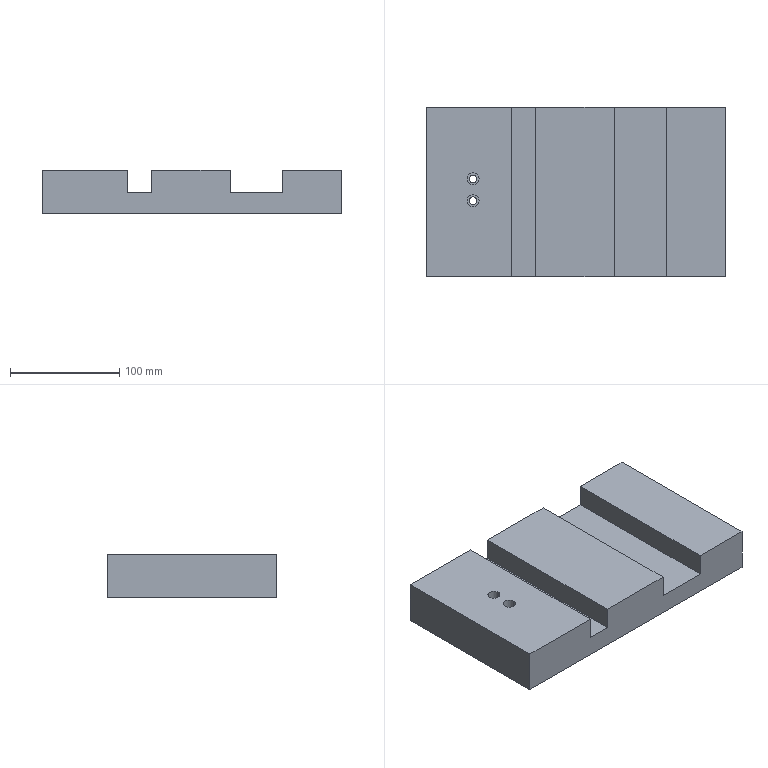Part | 1 solid | 24 faces | box 273.935 x 155 x 40 mm | volume 1471329 mm3 | plane 16 | cylinder 8 | commonest cylinder face diameters 7 x4 11 x4